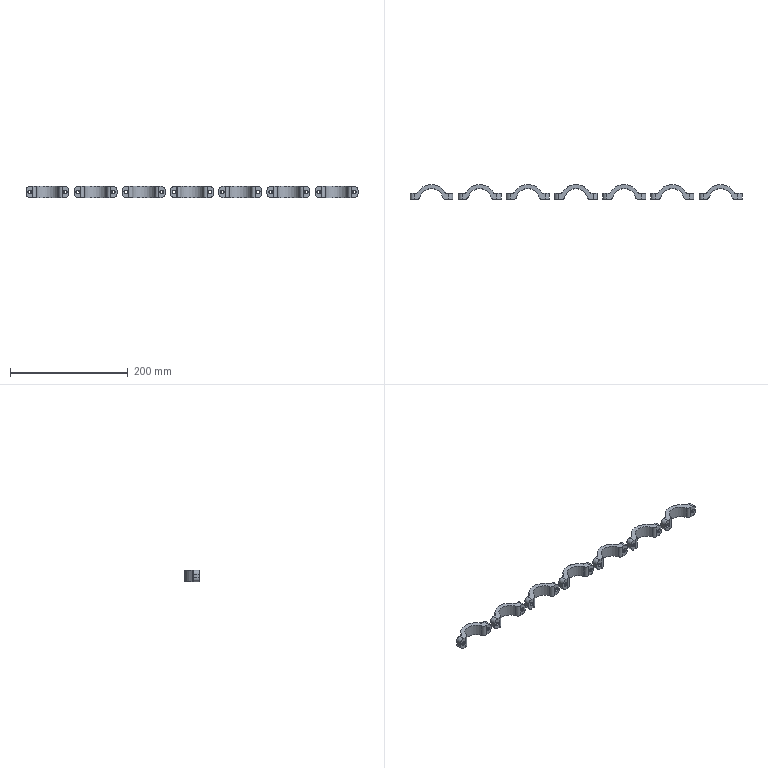NC program | Mastercam | posted with a generic post
Lines 19 to 689 of 23883:
(16 CO |TOOL - 1|DIA. OFF. - 1|LEN. - 1|TOOL DIA. - 16.)
N108 T1 M6
N110 G0 G56 G90 X59.5 Y-6.088 C0. B0. S5000 M3
N112 G43 H1 Z50.
N114 Z1.7
N116 G1 Z0. F2000.
N118 X29.5 F800.
N120 X27.235
N122 G2 X27.024 Y-6.09 I-.211 J13.302
N124 X25.198 Y-5.964 J13.304
N126 X23.929 Y-5.644 I1.236 J7.564
N128 G1 X22.899 Y-5.177
N130 X21.941 Y-4.5
N132 X21.15 Y-3.703
N134 G2 X20.028 Y-2.073 I9.785 J7.935
N136 G3 X-.005 Y9.09 I-20.033 J-12.394
N138 X-20.352 Y-2.596 J-23.557
N140 G2 X-21.648 Y-4.228 I-7.498 J4.62
N142 G1 X-22.536 Y-4.952
N144 X-23.578 Y-5.513
N146 X-24.662 Y-5.865
N148 X-25.746 Y-6.039
N150 G2 X-27.082 Y-6.089 I-1.336 J17.708
N152 X-27.243 Y-6.088 J17.758
N154 G1 X-29.5
N156 X-59.5
N158 G0 Z50.
N160 S6000 M3
N162 X-44.993 Y-23.147
N164 Z3.
N166 G1 Z-20.75 F2000.
N168 X-45.468 Y-21.965 Z-20.867 F4000.
N170 G3 X-46.263 Y-20.763 Z-21. I-3.341 J-1.344
N172 G1 X-46.694 Y-20.104
N174 G2 X-48.302 Y-14.728 I12.037 J6.529
N176 X-48.463 Y-10.938 I44.608 J3.79
N178 X-48.462 Y-10.646 I44.769
N180 G1 Y-10.633
N182 G2 X-48.44 Y-4.221 I934.293
N184 G1 X-48.437 Y-3.641
N186 X-48.348 Y12.996
N188 X-48.291 Y13.855
N190 G2 X-47.882 Y15.579 I8.002 J-.988
N192 X-46.124 Y18.512 I8.355 J-3.016
N194 X-42.668 Y21.033 I7.847 J-7.128
N196 X-39.623 Y22.037 I6.029 J-13.159
N198 X-35.754 Y22.54 I5.247 J-25.226
N200 X-30.718 Y22.676 I5.036 J-93.471
N202 X-30.105 Y22.674 J-93.607
N204 X-24.811 Y22.658 I-.005 J-896.025
N206 G1 X-24.226 Y22.655
N208 X34.366 Y22.355
N210 X34.575
N212 G2 X37.562 Y22.341 J-304.176
N214 X41.09 Y21.295 I-.512 J-8.198
N216 X44.287 Y18.474 I-5.158 J-9.067
N218 X46.399 Y14.335 I-11.41 J-8.434
N220 X47.292 Y10.36 I-21.593 J-6.94
N222 X47.718 Y4.959 I-53.145 J-6.907
N224 X47.842 Y-4.025 I-324.827 J-8.984
N226 G1 X47.841 Y-4.753
N228 X47.843 Y-5.348
N230 X47.849 Y-11.289
N232 G2 X47.853 Y-11.546 I-8.568 J-.257
N234 X47.766 Y-12.761 I-8.572
N236 X46.401 Y-16.232 I-8.475 J1.329
N238 X43.419 Y-19.18 I-8.921 J6.041
N240 X39.75 Y-20.926 I-8.089 J12.27
N242 X35.787 Y-21.802 I-6.913 J21.864
N244 X30.396 Y-22.22 I-6.893 J53.906
N246 X21.415 Y-22.342 I-8.981 J330.021
N248 G1 X20.687 Y-22.341
N250 X20.092 Y-22.343
N252 X-37.049 Y-22.34
N254 G2 X-41.217 Y-21.015 I.491 J8.76
N256 X-44.273 Y-18.125 I5.834 J9.228
N258 X-46.283 Y-14. I11.825 J8.316
N260 X-47.128 Y-10.041 I22.112 J6.79
N262 X-47.514 Y-4.653 I54.348 J6.599
N264 X-47.592 Y2.563 I332.574 J7.216
N266 X-47.583 Y5.054 I332.652
N268 G1 X-47.581 Y5.65
N270 X-47.563 Y9.588
N272 G2 X-44.702 Y16.72 I10.479 J-.065
N274 X-40.767 Y19.57 I9.439 J-8.889
N276 X-36.554 Y20.974 I7.861 J-16.565
N278 X-31.512 Y21.626 I6.969 J-34.093
N280 X-24.75 Y21.818 I6.762 J-118.83
N282 G1 X-24.599
N284 G2 X-21.261 Y21.824 I3.338 J-947.832
N286 X-15.636 Y21.807 J-947.838
N288 G1 X-15.042 Y21.804
N290 X34.051 Y21.552
N292 G2 X41.056 Y18.817 I-.316 J-11.149
N294 X44.279 Y14.675 I-8.967 J-10.301
N296 X45.905 Y10.179 I-16.992 J-8.688
N298 X46.673 Y5.154 I-33.963 J-7.761
N300 X46.982 Y-1.824 I-100.701 J-7.953
N302 X47.028 Y-7.263 I-322.601 J-5.439
N304 X47.024 Y-8.712 I-322.647
N306 X44.186 Y-15.691 I-11.146 J.466
N308 X43.363 Y-16.541 I-10.029 J8.886
N310 G3 X43.177 Y-16.761 I1.125 J-1.138
N312 G2 X41.844 Y-18.271 I-8.109 J5.821
N314 X37.061 Y-20.669 I-5.846 J5.69
N316 X29.843 Y-21.347 I-9.588 J63.352
N318 X20.091 Y-21.53 I-9.766 J259.865
N320 X18.3 Y-21.537 I-4.898 J995.578
N322 G1 X17.705 Y-21.539
N324 X-33.372 Y-21.549
N326 X-33.409
N328 G2 X-38.461 Y-20.369 J11.405
N330 G3 X-38.616 Y-20.307 I-.669 J-1.453
N332 G2 X-41.763 Y-18.351 I2.616 J7.719
N334 G1 X-42.182 Y-17.932
N336 G2 X-43.833 Y-15.677 I6.048 J6.16
N338 X-45.553 Y-11.213 I16.923 J9.081
N340 X-46.401 Y-6.131 I31.79 J7.918
N342 X-46.719 Y.296 I85.658 J7.46
N344 X-46.758 Y4.615 I237.547 J4.319
N346 X-46.744 Y7.207 I237.586
N348 X-45.393 Y12.515 I12.491 J-.354
N350 X-41.471 Y17.016 I11.507 J-6.067
N352 X-37.7 Y19.04 I9.641 J-13.438
N354 X-33.049 Y20.276 I8.514 J-22.663
N356 X-27.583 Y20.832 I7.594 J-47.54
N358 X-19.669 Y21.001 I7.914 J-185.44
N360 X-18.954 Y20.999 J-185.609
N362 X-17.61 Y21. I1.344 J-959.978
N364 X-14.176 Y20.994 J-959.979
N366 G1 X-13.581 Y20.992
N368 X30.998 Y20.764
N370 G2 X34.383 Y20.36 I-.104 J-15.255
N372 X40.858 Y16.504 I-3.087 J-12.549
N374 X43.539 Y12.46 I-11.725 J-10.683
N376 X45.095 Y7.782 I-20.436 J-9.394
N378 X45.882 Y2.198 I-40.212 J-8.516
N380 X46.178 Y-5.463 I-116.645 J-8.352
N382 G1 Y-5.57
N384 G2 X45.792 Y-8.923 I-14.719
N386 X44.787 Y-11.755 I-15.27 J3.824
N388 G3 X44.645 Y-12.362 I1.458 J-.66
N390 G2 X43.154 Y-16.795 I-8.145 J.274
N392 G3 X42.574 Y-18.114 Z-20.916 I2.939 J-2.078
N394 G1 X42.286 Y-19.447 Z-20.837
N396 G2 X41.951 Y-20.054 Z-20.797 I-1.173 J.253
N398 G1 X41.665 Y-20.333 Z-20.774
N400 G2 X41.329 Y-20.564 Z-20.75 I-.838 J.86
N402 X40.827 Y-20.674 Z-20.788 I-.502 J1.091
N404 X40.632 Y-20.658 Z-20.802 J1.201
N406 G1 X39.375 Y-20.45 Z-20.894
N408 G3 X38.79 Y-20.402 Z-20.937 I-.585 J-3.552
N410 X37.935 Y-20.505 Z-21. J-3.6
N412 G2 X35.824 Y-20.747 I-2.111 J9.071
N414 X35.407 Y-20.738 J9.313
N416 G1 X34.814
N418 X25.553
N420 X25.473
N422 G3 X22.169 Y-20.732 I-3.304 J-955.726
N424 X19.002 Y-20.738 J-955.732
N426 G1 X18.409 Y-20.739
N428 X-30.935
N430 G3 X-31.552 Y-20.737 I-.617 J-80.739
N432 X-32.145 Y-20.738 J-80.741
N434 G1 X-32.738
N436 X-36.
N438 G2 X-38.9 Y-20.205 J8.15
N440 G3 X-40.181 Y-19.969 Z-20.935 I-1.281 J-3.365
N442 X-43.272 Y-21.724 Z-20.75 J-3.601
N444 X-43.781 Y-23.57 I3.091 J-1.846 F9500.
N446 X-40.223 Y-27.169 I3.6
N448 G1 X25.396 Y-27.938
N450 X25.438
N452 G3 X29.038 Y-24.338 J3.6
N454 X28.989 Y-23.748 I-3.6
N456 X25.473 Y-20.738 Z-21. I-3.551 J-.59 F4000.
N458 G1 X24.88 Y-20.732
N460 G2 X22.208 Y-20.562 I.164 J23.583
N462 G1 X21.622 Y-20.468
N464 G3 X17.915 Y-20.102 I-4.508 J-26.73
N466 X10.314 Y-19.962 I-7.601 J-206.68
N468 X9.91 Y-19.963 J-206.82
N470 X8.732 Y-19.959 I-3.847 J-977.611
N472 G1 X8.142 Y-19.957
N474 X-19.27 Y-19.95
N476 G3 X-19.758 Y-20.026 J-1.6
N478 G2 X-22.913 Y-20.642 I-4.417 J14.244
N480 X-25.207 Y-20.741 I-2.294 J26.566
N482 X-25.553 Y-20.738 J26.665
N484 G1 X-26.146
N486 X-31.483
N488 G3 X-35.028 Y-23.713 Z-20.75 J-3.6
N490 X-35.083 Y-24.338 I3.545 J-.625 F9500.
N492 X-31.483 Y-27.938 I3.6
N494 G1 X-31.467
N496 X21.582 Y-27.705
N498 G3 X25.166 Y-24.105 I-.016 J3.6
N500 G1 Y-24.05
N502 G3 X22.137 Y-20.55 Z-21. I-3.6 J-.055 F4000.
N504 G2 X19.67 Y-19.993 I1.674 J13.162
N506 G3 X16.813 Y-19.507 I-4.185 J-15.956
N508 X11.419 Y-19.232 I-6.407 J-72.629
N510 X.38 Y-19.15 I-11.039 J-741.423
N512 X-1.483 Y-19.152 J-741.505
N514 G1 X-2.075
N516 X-16.782 Y-19.155
N518 G3 X-17.398 Y-19.174 I.263 J-18.436
N520 X-18.03 Y-19.335 I.069 J-1.599
N522 G2 X-19.794 Y-20.038 I-7.34 J15.855
N524 G3 X-22.31 Y-23.471 Z-20.774 I1.084 J-3.433
N526 X-22.279 Y-23.942 Z-20.75 I3.6
N528 X-18.733 Y-27.071 I3.569 J.471 F9500.
N530 G1 X19.538 Y-27.308
N532 X19.56
N534 G3 X23.144 Y-24.055 J3.6
N536 X23.161 Y-23.708 Z-20.767 I-3.584 J.347 F4000.
N538 X20.525 Y-20.24 Z-21. I-3.601
N540 G2 X19.109 Y-19.801 I4.302 J16.369
N542 X18.701 Y-19.631 I2.929 J7.606
N544 G3 X16.786 Y-19.078 I-3.562 J-8.757
N546 X12.937 Y-18.623 I-5.651 J-31.245
N548 X5.612 Y-18.395 I-7.881 J-135.55
N550 X-3.137 Y-18.355 I-8.749 J-954.021
N552 G1 X-3.217
N554 X-3.809 Y-18.354
N556 X-14.902 Y-18.365
N558 G3 X-16.222 Y-18.451 I.185 J-12.97
N560 X-16.861 Y-18.669 I.186 J-1.589
N562 G2 X-17.379 Y-18.98 I-227.845 J379.098
N564 X-18.591 Y-19.583 I-4.227 J6.981
N566 G3 X-20.861 Y-22.928 Z-20.787 I1.33 J-3.345
N568 X-20.786 Y-23.657 Z-20.75 I3.6
N570 X-17.306 Y-26.528 I3.525 J.729 F9500.
N572 G1 X18.379 Y-26.975
N574 X18.424
N576 G3 X21.989 Y-23.871 J3.6
N578 X22.023 Y-23.375 Z-20.775 I-3.565 J.496 F4000.
N580 X19.531 Y-19.95 Z-21. I-3.599
N582 G2 X17.593 Y-19.11 I4.809 J13.749
N584 G3 X15.762 Y-18.492 I-3.702 J-7.954
N586 X12.051 Y-17.939 I-5.816 J-26.309
N588 X5.414 Y-17.635 I-7.862 J-99.028
N590 X-7.13 Y-17.55 I-12.544 J-923.291
N592 X-9.283 Y-17.553 J-923.376
N594 G1 X-9.874 Y-17.552
N596 G3 X-10.641 Y-17.549 I-.767 J-107.594
N598 X-13.722 Y-17.594 J-107.597
N600 X-15.29 Y-17.752 I.364 J-11.471
N602 X-16. Y-18.073 I.284 J-1.574
N604 G2 X-16.87 Y-18.675 I-5.064 J6.387
N606 G3 X-18.618 Y-21.762 Z-20.816 I1.852 J-3.087
N608 X-18.38 Y-23.05 Z-20.75 I3.6
N610 X-15.132 Y-25.36 I3.362 J1.288 F9500.
N612 G1 X16.806 Y-26.376
N614 G3 X16.921 Y-26.378 I.115 J3.598
N616 X20.411 Y-23.659 J3.6
N618 X20.52 Y-22.778 Z-20.794 I-3.49 J.881 F4000.
N620 X18.395 Y-19.493 Z-21. I-3.599
N622 G2 X16.781 Y-18.622 I4.014 J9.368
N624 G3 X15.051 Y-17.94 I-3.786 J-7.072
N626 X11.486 Y-17.284 I-5.957 J-22.338
N628 X5.54 Y-16.899 I-7.648 J-72.007
N630 X-5.518 Y-16.761 I-11.058 J-443.515
N632 G1 X-6.122 Y-16.762
N634 X-6.712 Y-16.76
N636 G3 X-8.09 Y-16.755 I-1.378 J-193.906
N638 X-11.813 Y-16.791 J-193.911
N640 X-14.241 Y-17.011 I.197 J-15.697
N642 X-15.118 Y-17.333 I.249 J-2.028
N644 X-15.246 Y-17.434 I.924 J-1.307
N646 G2 X-16.232 Y-18.25 I-11.837 J13.314
N648 G3 X-17.698 Y-21.149 Z-20.832 I2.134 J-2.899
N650 X-17.324 Y-22.747 Z-20.75 I3.6
N652 X-14.244 Y-24.746 I3.226 J1.598 F9500.
N654 G1 X15.919 Y-25.971
N656 G3 X16.065 Y-25.974 I.146 J3.597
N658 X19.501 Y-23.447 J3.6
N660 X19.665 Y-22.374 Z-20.804 I-3.436 J1.073 F4000.
N662 X17.718 Y-19.176 Z-21. I-3.6
N664 G2 X16.008 Y-18.081 I7.121 J13.013
N666 G3 X13.93 Y-17.235 I-4.185 J-7.3
N668 X10.326 Y-16.551 I-6.307 J-23.385
N670 X3.832 Y-16.111 I-8.329 J-74.732
N672 X-6.277 Y-15.975 I-10.109 J-376.17
N674 X-10.012 Y-15.993 J-376.306
N676 X-13.132 Y-16.236 I.238 J-23.227
N678 X-13.924 Y-16.42 I1.162 J-6.792
N680 X-14.657 Y-16.866 I.434 J-1.54
N682 G2 X-15.308 Y-17.488 I-5.947 J5.572
N684 G3 X-16.569 Y-20.224 Z-20.845 I2.339 J-2.736
N686 X-16.07 Y-22.053 Z-20.75 I3.6
N688 X-13.147 Y-23.82 I3.101 J1.829 F9500.
N690 G1 X14.59 Y-25.194
N692 G3 X14.768 Y-25.198 I.178 J3.596
N694 X18.077 Y-23.017 J3.6
N696 X18.368 Y-21.598 Z-20.823 I-3.309 J1.419 F4000.
N698 X16.74 Y-18.586 Z-21. I-3.6
N700 G2 X15.55 Y-17.705 I4.778 J7.691
N702 G3 X14.128 Y-16.938 I-3.63 J-5.03
N704 X10.916 Y-16.067 I-5.988 J-15.729
N706 X5.797 Y-15.489 I-7.725 J-45.475
N708 X-2.737 Y-15.214 I-9.664 J-167.023
N710 X-5.72 Y-15.189 I-2.983 J-180.127
N712 X-8.981 Y-15.219 J-180.152
N714 X-12.181 Y-15.478 I.434 J-25.259
N716 X-13.464 Y-15.803 I1.057 J-6.866
N718 X-14.144 Y-16.275 I.542 J-1.505
N720 G2 X-14.779 Y-16.994 I-10.052 J8.252
N722 G3 X-15.805 Y-19.511 Z-20.861 I2.573 J-2.517
N724 X-15.132 Y-21.608 Z-20.75 I3.599
N726 X-12.435 Y-23.104 I2.926 J2.097 F9500.
N728 G1 X13.937 Y-24.788
N730 G3 X14.167 Y-24.795 I.23 J3.593
N732 X17.421 Y-22.733 J3.6
N734 X17.766 Y-21.195 Z-20.829 I-3.254 J1.538 F4000.
N736 X16.246 Y-18.257 Z-21. I-3.599
N738 G2 X14.99 Y-17.19 I6.042 J8.386
N740 G3 X13.253 Y-16.236 I-4.023 J-5.268
N742 X9.974 Y-15.34 I-6.353 J-16.8
N744 X4.855 Y-14.733 I-7.997 J-45.566
N746 X-5.139 Y-14.426 I-9.994 J-162.627
N748 X-8.084 Y-14.453 J-162.934
N750 X-11.323 Y-14.726 I.594 J-26.384
N752 X-12.975 Y-15.159 I1.054 J-7.395
N754 X-13.67 Y-15.691 I.588 J-1.488
N756 G2 X-14.779 Y-16.994 I-13.769 J10.603
N758 G3 X-15.805 Y-19.511 Z-20.861 I2.573 J-2.517
N760 X-15.132 Y-21.608 Z-20.75 I3.599
N762 X-12.348 Y-23.108 I2.926 J2.097 F9500.
N764 G1 X13.16 Y-24.118
N766 G3 X13.302 Y-24.121 I.142 J3.597
N768 X16.4 Y-22.356 J3.6
N770 X16.903 Y-20.521 Z-20.846 I-3.098 J1.835 F4000.
N772 X15.647 Y-17.789 Z-21. I-3.601
N774 G2 X14.421 Y-16.638 I11.895 J13.894
N776 G3 X12.71 Y-15.642 I-4.16 J-5.181
N778 X9.487 Y-14.687 I-6.5 J-16.01
N780 X4.43 Y-14.012 I-8.194 J-42.12
N782 X-4.72 Y-13.67 I-9.15 J-122.18
N784 X-7.236 Y-13.696 J-122.522
N786 X-10.902 Y-14.044 I.489 J-24.619
N788 X-12.597 Y-14.55 I1.169 J-7.002
N790 X-13.307 Y-15.162 I.644 J-1.465
N792 G2 X-13.98 Y-16.081 I-6.897 J4.342
N794 G3 X-14.83 Y-18.405 Z-20.874 I2.75 J-2.324
N796 X-13.997 Y-20.709 Z-20.75 I3.6
N798 X-11.472 Y-21.997 I2.767 J2.304 F9500.
N800 G1 X12.508 Y-23.613
N802 G3 X12.75 Y-23.621 I.242 J3.592
N804 X15.778 Y-21.967 J3.6
N806 X16.349 Y-20.021 Z-20.852 I-3.028 J1.946 F4000.
N808 X15.192 Y-17.377 Z-21. I-3.599
N810 G2 X14.165 Y-16.31 I5.985 J6.796
N812 G3 X12.758 Y-15.307 I-3.636 J-3.607
N814 X9.813 Y-14.222 I-6.286 J-12.522
N816 X4.961 Y-13.388 I-8.214 J-33.254
N818 X-4.326 Y-12.926 I-9.287 J-93.013
N820 X-6.51 Y-12.951 J-93.475
N822 X-10.201 Y-13.306 I.581 J-25.35
N824 X-12.036 Y-13.838 I1.4 J-8.259
N826 X-12.923 Y-14.544 I.613 J-1.681
N828 G1 X-13.236 Y-15.048
N830 G2 X-13.609 Y-15.608 I-7.881 J4.841
N832 G3 X-14.296 Y-17.723 Z-20.888 I2.914 J-2.115
N834 X-13.284 Y-20.224 Z-20.75 I3.601
N836 X-10.977 Y-21.312 I2.589 J2.501 F9500.
N838 G1 X11.941 Y-23.113
N840 G3 X12.223 Y-23.124 I.282 J3.589
N842 X15.179 Y-21.579 J3.6
N844 X15.823 Y-19.524 Z-20.859 I-2.956 J2.055 F4000.
N846 X14.76 Y-16.97 Z-21. I-3.6
N848 G2 X13.702 Y-15.718 I7.207 J7.158
N850 G3 X12.158 Y-14.632 I-4.136 J-4.24
N852 X9.159 Y-13.517 I-6.623 J-13.223
N854 X4.31 Y-12.651 I-8.46 J-33.366
N856 X-3.995 Y-12.196 I-8.305 J-75.537
N858 X-5.92 Y-12.22 J-75.992
N860 X-9.608 Y-12.586 I.637 J-25.181
N862 X-11.536 Y-13.14 I1.608 J-9.232
N864 X-11.948 Y-13.342 I1.842 J-4.275
N866 X-12.623 Y-14.018 I.743 J-1.417
N868 G2 X-13.278 Y-15.116 I-15.091 J8.256
N870 G3 X-13.818 Y-17.013 Z-20.901 I3.059 J-1.897
N872 X-12.619 Y-19.697 Z-20.75 I3.599
N874 X-10.502 Y-20.602 I2.4 J2.684 F9500.
N876 G1 X11.207 Y-22.315
N878 G3 X11.491 Y-22.326 I.284 J3.588
N880 X14.245 Y-21.045 J3.599
N882 X15.091 Y-18.727 Z-20.875 I-2.754 J2.318 F4000.
N884 X14.252 Y-16.417 Z-21. I-3.6
N886 G2 X13.308 Y-15.175 I15.909 J13.069
N888 G3 X11.771 Y-14.047 I-4.27 J-4.21
N890 X8.803 Y-12.88 I-6.785 J-12.898
N892 X4.004 Y-11.952 I-8.624 J-31.708
N894 X-3.673 Y-11.48 I-7.677 J-62.169
N896 X-5.531 Y-11.507 J-62.641
N898 X-9.18 Y-11.896 I.732 J-24.2
N900 X-11.367 Y-12.58 I1.667 J-9.16
N902 X-11.729 Y-12.781 I1.896 J-3.845
N904 X-12.449 Y-13.663 I.9 J-1.469
N906 G2 X-12.717 Y-14.191 I-7.399 J3.417
N908 G3 X-13.167 Y-15.934 Z-20.91 I3.15 J-1.743
N910 X-11.83 Y-18.734 Z-20.75 I3.6
N912 X-9.943 Y-19.514 I2.263 J2.8 F9500.
N914 G1 X10.616 Y-21.678
N916 G3 X10.993 Y-21.698 I.377 J3.58
N918 X13.661 Y-20.515 J3.6
N920 X14.593 Y-18.098 Z-20.882 I-2.668 J2.417 F4000.
N922 X13.836 Y-15.89 Z-21. I-3.6
N924 G2 X13.038 Y-14.77 I9.529 J7.632
N926 G3 X11.727 Y-13.657 I-3.83 J-3.185
N928 X8.958 Y-12.4 I-6.616 J-10.896
N930 X4.322 Y-11.345 I-8.615 J-27.132
N932 X-3.363 Y-10.78 I-7.685 J-51.976
N934 X-5.533 Y-10.824 J-52.541
N936 X-9.074 Y-11.275 I.948 J-21.572
N938 X-11.181 Y-12.012 I1.801 J-8.534
N940 X-11.922 Y-12.599 I.815 J-1.789
N942 X-12.091 Y-12.889 I1.289 J-.949
N944 G2 X-12.717 Y-14.191 I-23.545 J10.496
N946 G3 X-13.167 Y-15.934 Z-20.91 I3.15 J-1.743
N948 X-11.83 Y-18.734 Z-20.75 I3.6
N950 X-9.898 Y-19.519 I2.263 J2.8 F9500.
N952 G1 X10.441 Y-21.399
N954 G3 X10.773 Y-21.414 I.332 J3.585
N956 X13.428 Y-20.245 J3.6
N958 X14.373 Y-17.814 Z-20.883 I-2.655 J2.431 F4000.
N960 X13.628 Y-15.622 Z-21. I-3.6
N962 G2 X12.83 Y-14.396 I8.321 J6.289
N964 G3 X11.696 Y-13.287 I-3.733 J-2.682
N966 X9.121 Y-11.947 I-6.474 J-9.299
N968 X4.654 Y-10.764 I-8.581 J-23.371
N970 X-3.169 Y-10.09 I-7.823 J-45.061
N972 X-5.028 Y-10.127 J-45.735
N974 X-8.96 Y-10.662 I.851 J-20.98
N976 X-10.996 Y-11.439 I1.912 J-8.063
N978 X-11.704 Y-12.041 I.858 J-1.727
N980 X-11.885 Y-12.388 I1.318 J-.907
N982 G2 X-12.119 Y-12.949 I-7.633 J2.856
N984 G3 X-12.451 Y-14.458 Z-20.923 I3.268 J-1.509
N986 X-10.905 Y-17.415 Z-20.75 I3.6
N988 X-9.35 Y-18.023 I2.054 J2.957 F9500.
N990 G1 X9.793 Y-20.706
N992 G3 X10.292 Y-20.741 I.499 J3.566
N994 X12.769 Y-19.752 J3.601
N996 X13.892 Y-17.14 Z-20.895 I-2.477 J2.612 F4000.
N998 X13.295 Y-15.154 Z-21. I-3.6
N1000 G2 X12.56 Y-13.904 I12.901 J8.424
N1002 G3 X11.463 Y-12.768 I-3.878 J-2.645
N1004 X8.957 Y-11.379 I-6.539 J-8.845
N1006 X4.578 Y-10.125 I-8.611 J-21.808
N1008 X-2.961 Y-9.414 I-7.539 J-39.604
N1010 X-4.935 Y-9.463 J-40.315
N1012 X-8.796 Y-10.042 I.971 J-19.621
N1014 X-10.796 Y-10.852 I2.017 J-7.855
N1016 X-11.515 Y-11.489 I.963 J-1.811
N1018 X-11.679 Y-11.82 I1.341 J-.874
N1020 G2 X-12.119 Y-12.949 I-10.533 J3.451
N1022 G3 X-12.451 Y-14.458 Z-20.923 I3.268 J-1.509
N1024 X-10.905 Y-17.415 Z-20.75 I3.6
N1026 X-9.268 Y-18.034 I2.054 J2.957 F9500.
N1028 G1 X9.572 Y-20.235
N1030 G3 X9.99 Y-20.259 I.418 J3.575
N1032 X12.364 Y-19.366 J3.599
N1034 X13.59 Y-16.66 Z-20.902 I-2.374 J2.706 F4000.
N1036 X13.067 Y-14.791 Z-21. I-3.6
N1038 G2 X12.316 Y-13.399 I12.138 J7.449
N1040 G3 X11.21 Y-12.211 I-4.087 J-2.697
N1042 X8.725 Y-10.777 I-6.621 J-8.596
N1044 X4.399 Y-9.472 I-8.644 J-20.835
N1046 X-2.776 Y-8.751 I-7.175 J-35.362
N1048 X-4.948 Y-8.817 J-36.083
N1050 X-8.716 Y-9.45 I1.12 J-18.188
N1052 X-10.659 Y-10.297 I2.111 J-7.497
N1054 X-11.318 Y-10.918 I.951 J-1.669
N1056 X-11.47 Y-11.238 I1.36 J-.843
N1058 G2 X-11.852 Y-12.298 I-79.076 J27.869
N1060 G3 X-12.065 Y-13.519 Z-20.938 I3.387 J-1.221
N1062 X-10.256 Y-16.642 Z-20.75 I3.6
N1064 X-8.936 Y-17.088 I1.791 J3.123 F9500.
N1066 G1 X9.073 Y-19.461
N1068 G3 X9.544 Y-19.492 I.471 J3.569
N1070 X11.769 Y-18.722 J3.6
N1072 X13.144 Y-15.892 Z-20.912 I-2.225 J2.83 F4000.
N1074 X12.717 Y-14.192 Z-21. I-3.6
N1076 G2 X12.136 Y-12.996 I13.671 J7.382
N1078 G3 X11.193 Y-11.843 I-3.714 J-2.075
N1080 X8.882 Y-10.348 I-6.425 J-7.399
N1082 X4.716 Y-8.932 I-8.58 J-18.408
N1084 X-2.617 Y-8.098 I-7.333 J-31.833
N1086 X-4.944 Y-8.181 J-32.667
N1088 X-8.636 Y-8.863 I1.246 J-17.075
N1090 X-10.519 Y-9.736 I2.177 J-7.165
N1092 X-11.273 Y-10.652 I.928 J-1.532
N1094 G2 X-11.708 Y-11.899 I-32.76 J10.732
N1096 G3 X-11.922 Y-13.121 Z-20.938 I3.386 J-1.222
N1098 X-10.113 Y-16.243 Z-20.75 I3.6
N1100 X-8.813 Y-16.687 I1.791 J3.122 F9500.
N1102 G1 X8.879 Y-19.124
N1104 G3 X9.37 Y-19.158 I.491 J3.566
N1106 X11.55 Y-18.422 J3.6
N1108 X12.969 Y-15.558 Z-20.915 I-2.18 J2.864 F4000.
N1110 X12.57 Y-13.908 Z-21. I-3.599
N1112 G2 X11.899 Y-12.433 I12.845 J6.728
N1114 G3 X10.902 Y-11.219 I-4.011 J-2.279
N1116 X8.567 Y-9.695 I-6.639 J-7.621
N1118 X4.419 Y-8.26 I-8.599 J-18.14
N1120 X-2.51 Y-7.455 I-6.929 J-29.432
N1122 X-4.645 Y-7.531 J-30.237
N1124 X-8.334 Y-8.208 I1.218 J-17.03
N1126 X-10.265 Y-9.092 I2.273 J-7.514
N1128 X-10.998 Y-9.917 I.91 J-1.547
N1130 X-11.507 Y-11.341 I15.372 J-6.293
N1132 G1 X-11.708 Y-11.899
N1134 G3 X-11.922 Y-13.121 Z-20.938 I3.386 J-1.222
N1136 X-10.113 Y-16.243 Z-20.75 I3.6
N1138 X-8.684 Y-16.702 I1.791 J3.122 F9500.
N1140 G1 X8.671 Y-18.46
N1142 G3 X9.033 Y-18.478 I.362 J3.582
N1144 X11.079 Y-17.84 J3.6
N1146 X12.633 Y-14.878 Z-20.923 I-2.046 J2.962 F4000.
N1148 X12.306 Y-13.377 Z-21. I-3.6
N1150 G2 X11.693 Y-11.879 I28.482 J12.514
N1152 G3 X10.644 Y-10.603 I-4.301 J-2.469
N1154 X8.288 Y-9.05 I-6.837 J-7.809
N1156 X4.163 Y-7.599 I-8.584 J-17.815
N1158 X-2.384 Y-6.823 I-6.547 J-27.236
N1160 X-4.768 Y-6.925 J-28.012
N1162 X-8.361 Y-7.662 I1.38 J-15.857
N1164 X-10.105 Y-8.512 I2.267 J-6.866
N1166 X-10.63 Y-9.113 I.904 J-1.32
N1168 X-11.234 Y-10.536 I10.598 J-5.334
N1170 X-11.422 Y-11.684 Z-20.942 I3.412 J-1.148
N1172 X-9.545 Y-14.845 Z-20.75 I3.6
N1174 X-8.34 Y-15.246 I1.723 J3.161 F9500.
N1176 G1 X8.178 Y-17.648
N1178 G3 X8.696 Y-17.685 I.518 J3.562
N1180 X10.633 Y-17.12 J3.599
N1182 X12.296 Y-14.086 Z-20.93 I-1.937 J3.034 F4000.
N1184 X12.021 Y-12.705 Z-21. I-3.6
N1186 G2 X11.519 Y-11.369 I12.517 J5.464
N1188 G3 X10.499 Y-10.076 I-4.319 J-2.357
N1190 X8.193 Y-8.491 I-6.873 J-7.533
N1192 X3.693 Y-6.89 I-8.663 J-17.217
N1194 X-2.285 Y-6.199 I-5.978 J-25.502
N1196 X-4.668 Y-6.307 J-26.193
N1198 X-8.229 Y-7.066 I1.414 J-15.377
N1200 X-9.637 Y-7.73 I2.284 J-6.662
N1202 X-10.15 Y-8.249 I.852 J-1.354
N1204 X-10.962 Y-9.83 I10.15 J-6.213
N1206 X-11.246 Y-11.231 Z-20.928 I3.316 J-1.401
N1208 X-9.601 Y-14.254 Z-20.75 I3.6
N1210 X-8.155 Y-14.795 I1.955 J3.023 F9500.
N1212 G1 X7.959 Y-17.097
N1214 G3 X8.468 Y-17.133 I.509 J3.564
N1216 X10.355 Y-16.599 J3.6
N1218 X12.068 Y-13.533 Z-20.932 I-1.887 J3.066 F4000.
N1220 X11.815 Y-12.208 Z-21. I-3.6
N1222 G2 X11.327 Y-10.808 I29.403 J11.047
N1224 G3 X10.3 Y-9.487 I-4.412 J-2.368
N1226 X7.644 Y-7.695 I-7.137 J-7.718
N1228 X3.082 Y-6.154 I-8.55 J-17.792
N1230 X-2.198 Y-5.582 I-5.28 J-24.099
N1232 X-4.718 Y-5.712 J-24.671
N1234 X-8.188 Y-6.508 I1.496 J-14.492
N1236 X-8.974 Y-6.864 I2.476 J-6.5
N1238 X-9.526 Y-7.33 I.729 J-1.425
N1240 X-10.482 Y-8.828 I9.526 J-7.132
N1242 X-10.911 Y-10.532 Z-20.912 I3.171 J-1.704
N1244 X-9.54 Y-13.359 Z-20.75 I3.6
N1246 X-7.835 Y-14.094 I2.229 J2.827 F9500.
N1248 G1 X7.685 Y-16.377
N1250 G3 X8.209 Y-16.415 I.524 J3.562
N1252 X9.948 Y-15.967 J3.6
N1254 X11.809 Y-12.815 Z-20.941 I-1.739 J3.152 F4000.
N1256 X11.615 Y-11.65 Z-21. I-3.6
N1258 G1 X11.327 Y-10.808
N1260 G3 X10.473 Y-9.287 I-3.52 J-.975
N1262 X8.456 Y-7.635 I-6.409 J-5.769
N1264 X4.662 Y-5.976 I-8.406 J-14.056
N1266 X-2.148 Y-4.975 I-6.81 J-22.67
N1268 X-4.365 Y-5.079 J-23.671
N1270 X-7.809 Y-5.83 I1.336 J-14.401
N1272 X-8.196 Y-5.991 I2.255 J-5.983
N1274 X-8.722 Y-6.366 I.647 J-1.463
N1276 X-10.152 Y-8.253 I8.722 J-8.096
N1278 X-10.681 Y-10.131 Z-20.902 I3.071 J-1.878
N1280 X-9.464 Y-12.83 Z-20.75 I3.6
N1282 X-7.602 Y-13.693 I2.383 J2.699 F9500.
N1284 G1 X7.527 Y-15.908
N1286 G3 X8.048 Y-15.946 I.521 J3.562
N1288 X9.787 Y-15.498 J3.6
N1290 X11.648 Y-12.346 Z-20.941 I-1.739 J3.152 F4000.
N1292 X11.455 Y-11.181 Z-21. I-3.6
N1294 X10.809 Y-9.484 I-14.707 J-4.624
N1296 X9.729 Y-8.136 I-4.634 J-2.604
N1298 X7.033 Y-6.343 I-7.293 J-8.047
N1300 X2.057 Y-4.758 I-8.389 J-17.728
N1302 X-2.055 Y-4.372 I-4.112 J-21.709
N1304 X-4.675 Y-4.528 J-22.095
N1306 X-7.149 Y-5.072 I1.57 J-13.03
N1308 X-7.675 Y-5.367 I.506 J-1.518
N1310 X-9.323 Y-7.067 I7.675 J-9.095
N1312 X-10.103 Y-9.304 Z-20.88 I2.82 J-2.237
N1314 X-9.196 Y-11.693 Z-20.75 I3.6
N1316 X-7.065 Y-12.86 I2.693 J2.389 F9500.
N1318 G1 X7.215 Y-15.118
N1320 G3 X7.777 Y-15.162 I.562 J3.555
N1322 X9.601 Y-14.666 J3.599
N1324 X11.376 Y-11.563 Z-20.936 I-1.824 J3.103 F4000.
N1326 G1 X11.351 Y-11.136 Z-20.957
N1328 X11.275 Y-10.715 Z-20.979
N1330 X11.15 Y-10.306 Z-21.
N1332 G3 X10.26 Y-8.434 I-11.151 J-4.157
N1334 X8.672 Y-6.837 I-5.586 J-3.966
N1336 X5.21 Y-5.03 I-8.043 J-11.196
N1338 X-2.013 Y-3.781 I-7.223 J-20.256
N1340 X-4.428 Y-3.917 J-21.505
N1342 X-5.797 Y-4.157 I1.537 J-12.809
N1344 X-6.289 Y-4.359 I.354 J-1.56
N1346 X-8.164 Y-5.804 I6.289 J-10.103
N1348 X-9.294 Y-8.423 Z-20.854 I2.469 J-2.619
N1350 X-8.703 Y-10.401 Z-20.75 I3.599
N1352 X-6.336 Y-11.965 I3.008 J1.978 F9500.
N1354 G1 X6.809 Y-14.346
N1356 G3 X7.45 Y-14.404 I.641 J3.543
N1358 X9.574 Y-13.71 J3.601
N1360 X11.05 Y-10.803 Z-20.918 I-2.124 J2.907 F4000.
N1362 X10.682 Y-9.217 Z-21. I-3.6
N1364 X9.369 Y-7.136 I-10.101 J-4.917
N1366 X7.437 Y-5.568 I-5.878 J-5.267
N1368 X3.267 Y-3.866 I-7.98 J-13.6
N1370 X-1.945 Y-3.192 I-5.212 J-19.806
N1372 X-3.952 Y-3.291 J-20.48
N1374 X-4.373 Y-3.394 I.167 J-1.591
N1376 X-6.967 Y-4.814 I4.373 J-11.068
N1378 X-8.46 Y-7.733 Z-20.831 I2.108 J-2.919
N1380 X-8.099 Y-9.302 Z-20.75 I3.601
N1382 X-5.532 Y-11.269 I3.24 J1.569 F9500.
N1384 G1 X6.317 Y-13.521
N1386 G3 X6.989 Y-13.584 I.672 J3.536
N1388 X9.428 Y-12.633 J3.599
N1390 X10.589 Y-9.985 Z-20.898 I-2.439 J2.648 F4000.
N1392 X10.021 Y-8.043 Z-21. I-3.6
N1394 X7.687 Y-5.388 I-9.53 J-6.023
N1396 X4.841 Y-3.836 I-6.716 J-8.929
N1398 X-1.11 Y-2.631 I-6.741 J-17.995
N1400 X-1.951 Y-2.723 I.001 J-3.921
N1402 X-5.322 Y-3.818 I1.951 J-11.739
N1404 X-7.312 Y-7.038 Z-20.802 I1.61 J-3.22
N1406 X-7.163 Y-8.065 Z-20.75 I3.6
N1408 X-4.318 Y-10.587 I3.451 J1.027 F9500.
N1410 G1 X5.359 Y-12.238
N1412 G3 X5.964 Y-12.289 I.605 J3.549
N1414 X8.879 Y-10.802 J3.6
N1416 X9.564 Y-8.689 Z-20.862 I-2.915 J2.113 F4000.
N1418 X8.551 Y-6.186 Z-21. I-3.6
N1420 X0. Y-2.562 I-8.551 J-8.276
N1422 X-2.012 Y-2.733 J-11.9
N1424 X-4.343 Y-4.202 Z-20.859 I.609 J-3.548
N1426 G1 X-4.798 Y-4.846 Z-20.82
N1428 G3 X-5.551 Y-6.038 Z-20.75 I11.166 J-7.896
N1430 X-6.599 Y-8.399 I11.919 J-6.704 F9500.
N1432 G1 X-8.161 Y-13.062
N1434 G2 X-16.415 Y-21.556 I-12.967 J4.343
N1436 X-17.454 Y-21.854 I-2.587 J7.047
N1438 G1 X-33.355 Y-25.207
N1440 G2 X-34.903 Y-25.368 I-1.548 J7.346
N1442 X-41.442 Y-21.548 J7.507
N1444 X-42.229 Y-19.499 Z-20.86 I6.539 J3.687 F4000.
N1446 G1 X-42.529 Y-18.159 Z-20.928